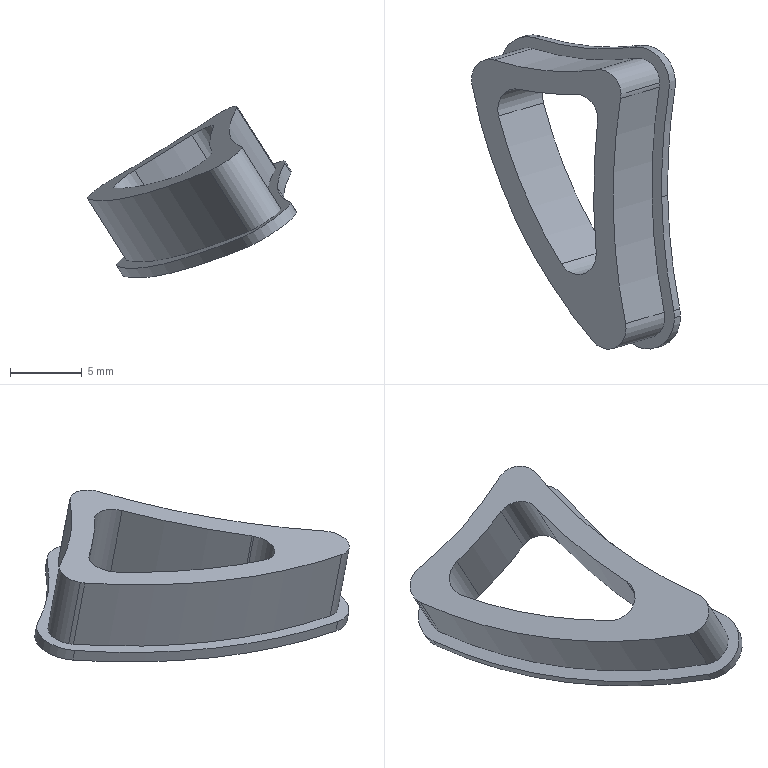Part | SolidWorks | features SplitBody 1 | 1 solid | 26 faces | box 14.584 x 21.952 x 12.002 mm | volume 557.744 mm3 | cylinder 23 | plane 3 | commonest cylinder face diameters 3.2 x9 4.8 x4 78.4 x2 43.2 x1 44.8 x1 48 x1
STEP:
#1=CARTESIAN_POINT('',(533.227,266.339,-385.084));
#2=VERTEX_POINT('',#1);
#3=CARTESIAN_POINT('',(533.176,266.825,-385.025));
#4=VERTEX_POINT('',#3);
#5=CARTESIAN_POINT('',(531.189,266.525,-386.337));
#6=DIRECTION('',(-0.5274,-0.157,0.835));
#7=DIRECTION('',(-0.8494,0.07732,-0.522));
#8=AXIS2_PLACEMENT_3D('',#5,#6,#7);
#9=CIRCLE('',#8,2.4);
#10=EDGE_CURVE('',#2,#4,#9,.T.);
#11=ORIENTED_EDGE('',*,*,#10,.F.);
#12=CARTESIAN_POINT('',(533.649,266.465,-385.752));
#13=VERTEX_POINT('',#12);
#14=CARTESIAN_POINT('',(533.649,266.465,-385.752));
#15=DIRECTION('',(0.5274,0.157,-0.835));
#16=VECTOR('',#15,1000.);
#17=LINE('',#14,#16);
#18=EDGE_CURVE('',#2,#13,#17,.T.);
#19=ORIENTED_EDGE('',*,*,#18,.T.);
#20=CARTESIAN_POINT('',(533.598,266.95,-385.693));
#21=VERTEX_POINT('',#20);
#22=CARTESIAN_POINT('',(531.611,266.65,-387.005));
#23=DIRECTION('',(0.5274,0.157,-0.835));
#24=DIRECTION('',(-0.8494,0.07732,-0.522));
#25=AXIS2_PLACEMENT_3D('',#22,#23,#24);
#26=CIRCLE('',#25,2.4);
#27=EDGE_CURVE('',#21,#13,#26,.T.);
#28=ORIENTED_EDGE('',*,*,#27,.F.);
#29=CARTESIAN_POINT('',(533.598,266.95,-385.693));
#30=DIRECTION('',(0.5274,0.157,-0.835));
#31=VECTOR('',#30,1000.);
#32=LINE('',#29,#31);
#33=EDGE_CURVE('',#4,#21,#32,.T.);
#34=ORIENTED_EDGE('',*,*,#33,.F.);
#35=EDGE_LOOP('',(#11,#19,#28,#34));
#36=FACE_OUTER_BOUND('',#35,.T.);
#37=CARTESIAN_POINT('',(531.611,266.65,-387.005));
#38=DIRECTION('',(0.5274,0.157,-0.835));
#39=DIRECTION('',(0.8494,-0.07732,0.522));
#40=AXIS2_PLACEMENT_3D('',#37,#38,#39);
#41=CYLINDRICAL_SURFACE('',#40,2.4);
#42=ADVANCED_FACE('',(#36),#41,.T.);
#43=CARTESIAN_POINT('',(529.493,281.935,-378.378));
#44=VERTEX_POINT('',#43);
#45=CARTESIAN_POINT('',(527.854,283.63,-379.094));
#46=VERTEX_POINT('',#45);
#47=CARTESIAN_POINT('',(528.134,282.059,-379.213));
#48=DIRECTION('',(-0.5274,-0.157,0.835));
#49=DIRECTION('',(-0.8494,0.07732,-0.522));
#50=AXIS2_PLACEMENT_3D('',#47,#48,#49);
#51=CIRCLE('',#50,1.6);
#52=EDGE_CURVE('',#44,#46,#51,.T.);
#53=ORIENTED_EDGE('',*,*,#52,.F.);
#54=CARTESIAN_POINT('',(532.193,282.739,-382.653));
#55=VERTEX_POINT('',#54);
#56=CARTESIAN_POINT('',(529.493,281.935,-378.378));
#57=DIRECTION('',(0.5274,0.157,-0.835));
#58=VECTOR('',#57,1000.);
#59=LINE('',#56,#58);
#60=EDGE_CURVE('',#44,#55,#59,.T.);
#61=ORIENTED_EDGE('',*,*,#60,.T.);
#62=CARTESIAN_POINT('',(530.555,284.434,-383.369));
#63=VERTEX_POINT('',#62);
#64=CARTESIAN_POINT('',(530.834,282.863,-383.488));
#65=DIRECTION('',(0.5274,0.157,-0.835));
#66=DIRECTION('',(-0.8494,0.07732,-0.522));
#67=AXIS2_PLACEMENT_3D('',#64,#65,#66);
#68=CIRCLE('',#67,1.6);
#69=EDGE_CURVE('',#63,#55,#68,.T.);
#70=ORIENTED_EDGE('',*,*,#69,.F.);
#71=CARTESIAN_POINT('',(527.854,283.63,-379.094));
#72=DIRECTION('',(0.5274,0.157,-0.835));
#73=VECTOR('',#72,1000.);
#74=LINE('',#71,#73);
#75=EDGE_CURVE('',#46,#63,#74,.T.);
#76=ORIENTED_EDGE('',*,*,#75,.F.);
#77=EDGE_LOOP('',(#53,#61,#70,#76));
#78=FACE_OUTER_BOUND('',#77,.T.);
#79=CARTESIAN_POINT('',(528.134,282.059,-379.213));
#80=DIRECTION('',(0.5274,0.157,-0.835));
#81=DIRECTION('',(0.8494,-0.07732,0.522));
#82=AXIS2_PLACEMENT_3D('',#79,#80,#81);
#83=CYLINDRICAL_SURFACE('',#82,1.6);
#84=ADVANCED_FACE('',(#78),#83,.T.);
#85=CARTESIAN_POINT('',(521.766,283.72,-389.055));
#86=VERTEX_POINT('',#85);
#87=CARTESIAN_POINT('',(523.36,285.118,-387.786));
#88=VERTEX_POINT('',#87);
#89=CARTESIAN_POINT('',(523.125,283.596,-388.22));
#90=DIRECTION('',(0.5274,0.157,-0.835));
#91=DIRECTION('',(-0.8494,0.07732,-0.522));
#92=AXIS2_PLACEMENT_3D('',#89,#90,#91);
#93=CIRCLE('',#92,1.6);
#94=EDGE_CURVE('',#86,#88,#93,.T.);
#95=ORIENTED_EDGE('',*,*,#94,.F.);
#96=CARTESIAN_POINT('',(519.066,282.916,-384.78));
#97=VERTEX_POINT('',#96);
#98=CARTESIAN_POINT('',(519.066,282.916,-384.78));
#99=DIRECTION('',(-0.5274,-0.157,0.835));
#100=VECTOR('',#99,1000.);
#101=LINE('',#98,#100);
#102=EDGE_CURVE('',#86,#97,#101,.T.);
#103=ORIENTED_EDGE('',*,*,#102,.T.);
#104=CARTESIAN_POINT('',(520.659,284.314,-383.511));
#105=VERTEX_POINT('',#104);
#106=CARTESIAN_POINT('',(520.425,282.792,-383.945));
#107=DIRECTION('',(-0.5274,-0.157,0.835));
#108=DIRECTION('',(-0.8494,0.07732,-0.522));
#109=AXIS2_PLACEMENT_3D('',#106,#107,#108);
#110=CIRCLE('',#109,1.6);
#111=EDGE_CURVE('',#105,#97,#110,.T.);
#112=ORIENTED_EDGE('',*,*,#111,.F.);
#113=CARTESIAN_POINT('',(520.659,284.314,-383.511));
#114=DIRECTION('',(-0.5274,-0.157,0.835));
#115=VECTOR('',#114,1000.);
#116=LINE('',#113,#115);
#117=EDGE_CURVE('',#88,#105,#116,.T.);
#118=ORIENTED_EDGE('',*,*,#117,.F.);
#119=EDGE_LOOP('',(#95,#103,#112,#118));
#120=FACE_OUTER_BOUND('',#119,.T.);
#121=CARTESIAN_POINT('',(520.425,282.792,-383.945));
#122=DIRECTION('',(-0.5274,-0.157,0.835));
#123=DIRECTION('',(-0.8494,0.07732,-0.522));
#124=AXIS2_PLACEMENT_3D('',#121,#122,#123);
#125=CYLINDRICAL_SURFACE('',#124,1.6);
#126=ADVANCED_FACE('',(#120),#125,.T.);
#127=CARTESIAN_POINT('',(527.769,270.804,-381.56));
#128=VERTEX_POINT('',#127);
#129=CARTESIAN_POINT('',(525.33,270.097,-383.234));
#130=VERTEX_POINT('',#129);
#131=CARTESIAN_POINT('',(526.41,270.928,-382.395));
#132=DIRECTION('',(0.5274,0.157,-0.835));
#133=DIRECTION('',(-0.8494,0.07732,-0.522));
#134=AXIS2_PLACEMENT_3D('',#131,#132,#133);
#135=CIRCLE('',#134,1.6);
#136=EDGE_CURVE('',#128,#130,#135,.T.);
#137=ORIENTED_EDGE('',*,*,#136,.F.);
#138=CARTESIAN_POINT('',(530.892,271.733,-386.503));
#139=VERTEX_POINT('',#138);
#140=CARTESIAN_POINT('',(527.769,270.804,-381.56));
#141=DIRECTION('',(0.5274,0.157,-0.835));
#142=VECTOR('',#141,1000.);
#143=LINE('',#140,#142);
#144=EDGE_CURVE('',#128,#139,#143,.T.);
#145=ORIENTED_EDGE('',*,*,#144,.T.);
#146=CARTESIAN_POINT('',(528.452,271.027,-388.177));
#147=VERTEX_POINT('',#146);
#148=CARTESIAN_POINT('',(529.533,271.857,-387.338));
#149=DIRECTION('',(-0.5274,-0.157,0.835));
#150=DIRECTION('',(-0.8494,0.07732,-0.522));
#151=AXIS2_PLACEMENT_3D('',#148,#149,#150);
#152=CIRCLE('',#151,1.6);
#153=EDGE_CURVE('',#147,#139,#152,.T.);
#154=ORIENTED_EDGE('',*,*,#153,.F.);
#155=CARTESIAN_POINT('',(525.33,270.097,-383.234));
#156=DIRECTION('',(0.5274,0.157,-0.835));
#157=VECTOR('',#156,1000.);
#158=LINE('',#155,#157);
#159=EDGE_CURVE('',#130,#147,#158,.T.);
#160=ORIENTED_EDGE('',*,*,#159,.F.);
#161=EDGE_LOOP('',(#137,#145,#154,#160));
#162=FACE_OUTER_BOUND('',#161,.T.);
#163=CARTESIAN_POINT('',(526.41,270.928,-382.395));
#164=DIRECTION('',(0.5274,0.157,-0.835));
#165=DIRECTION('',(0.8494,-0.07732,0.522));
#166=AXIS2_PLACEMENT_3D('',#163,#164,#165);
#167=CYLINDRICAL_SURFACE('',#166,1.6);
#168=ADVANCED_FACE('',(#162),#167,.F.);
#169=CARTESIAN_POINT('',(532.759,274.886,-384.731));
#170=VERTEX_POINT('',#169);
#171=CARTESIAN_POINT('',(566.056,271.855,-364.267));
#172=DIRECTION('',(0.5274,0.157,-0.835));
#173=DIRECTION('',(-0.8494,0.07732,-0.522));
#174=AXIS2_PLACEMENT_3D('',#171,#172,#173);
#175=CIRCLE('',#174,39.2);
#176=EDGE_CURVE('',#21,#170,#175,.T.);
#177=ORIENTED_EDGE('',*,*,#176,.T.);
#178=CARTESIAN_POINT('',(532.337,274.761,-384.063));
#179=VERTEX_POINT('',#178);
#180=CARTESIAN_POINT('',(532.759,274.886,-384.731));
#181=DIRECTION('',(-0.5274,-0.157,0.835));
#182=VECTOR('',#181,1000.);
#183=LINE('',#180,#182);
#184=EDGE_CURVE('',#170,#179,#183,.T.);
#185=ORIENTED_EDGE('',*,*,#184,.T.);
#186=CARTESIAN_POINT('',(565.634,271.73,-363.599));
#187=DIRECTION('',(0.5274,0.157,-0.835));
#188=DIRECTION('',(-0.8494,0.07732,-0.522));
#189=AXIS2_PLACEMENT_3D('',#186,#187,#188);
#190=CIRCLE('',#189,39.2);
#191=EDGE_CURVE('',#4,#179,#190,.T.);
#192=ORIENTED_EDGE('',*,*,#191,.F.);
#193=ORIENTED_EDGE('',*,*,#33,.T.);
#194=EDGE_LOOP('',(#177,#185,#192,#193));
#195=FACE_OUTER_BOUND('',#194,.T.);
#196=CARTESIAN_POINT('',(566.056,271.855,-364.267));
#197=DIRECTION('',(-0.5274,-0.157,0.835));
#198=DIRECTION('',(-0.8494,0.07732,-0.522));
#199=AXIS2_PLACEMENT_3D('',#196,#197,#198);
#200=CYLINDRICAL_SURFACE('',#199,39.2);
#201=ADVANCED_FACE('',(#195),#200,.F.);
#202=CARTESIAN_POINT('',(519.099,282.597,-384.819));
#203=VERTEX_POINT('',#202);
#204=CARTESIAN_POINT('',(527.566,264.672,-382.842));
#205=VERTEX_POINT('',#204);
#206=CARTESIAN_POINT('',(546.94,286.701,-366.461));
#207=DIRECTION('',(-0.5274,-0.157,0.835));
#208=DIRECTION('',(-0.8494,0.07732,-0.522));
#209=AXIS2_PLACEMENT_3D('',#206,#207,#208);
#210=CIRCLE('',#209,33.6);
#211=EDGE_CURVE('',#203,#205,#210,.T.);
#212=ORIENTED_EDGE('',*,*,#211,.F.);
#213=CARTESIAN_POINT('',(521.8,283.401,-389.094));
#214=VERTEX_POINT('',#213);
#215=CARTESIAN_POINT('',(519.099,282.597,-384.819));
#216=DIRECTION('',(0.5274,0.157,-0.835));
#217=VECTOR('',#216,1000.);
#218=LINE('',#215,#217);
#219=EDGE_CURVE('',#203,#214,#218,.T.);
#220=ORIENTED_EDGE('',*,*,#219,.T.);
#221=CARTESIAN_POINT('',(530.266,265.476,-387.117));
#222=VERTEX_POINT('',#221);
#223=CARTESIAN_POINT('',(549.64,287.505,-370.736));
#224=DIRECTION('',(-0.5274,-0.157,0.835));
#225=DIRECTION('',(-0.8494,0.07732,-0.522));
#226=AXIS2_PLACEMENT_3D('',#223,#224,#225);
#227=CIRCLE('',#226,33.6);
#228=EDGE_CURVE('',#214,#222,#227,.T.);
#229=ORIENTED_EDGE('',*,*,#228,.T.);
#230=CARTESIAN_POINT('',(527.566,264.672,-382.842));
#231=DIRECTION('',(-0.5274,-0.157,0.835));
#232=VECTOR('',#231,1000.);
#233=LINE('',#230,#232);
#234=EDGE_CURVE('',#222,#205,#233,.T.);
#235=ORIENTED_EDGE('',*,*,#234,.T.);
#236=EDGE_LOOP('',(#212,#220,#229,#235));
#237=FACE_OUTER_BOUND('',#236,.T.);
#238=CARTESIAN_POINT('',(546.94,286.701,-366.461));
#239=DIRECTION('',(0.5274,0.157,-0.835));
#240=DIRECTION('',(0.8494,-0.07732,0.522));
#241=AXIS2_PLACEMENT_3D('',#238,#239,#240);
#242=CYLINDRICAL_SURFACE('',#241,33.6);
#243=ADVANCED_FACE('',(#237),#242,.T.);
#244=CARTESIAN_POINT('',(532.514,266.725,-385.462));
#245=VERTEX_POINT('',#244);
#246=CARTESIAN_POINT('',(532.173,282.435,-382.723));
#247=VERTEX_POINT('',#246);
#248=CARTESIAN_POINT('',(565.634,271.73,-363.599));
#249=DIRECTION('',(0.5274,0.157,-0.835));
#250=DIRECTION('',(-0.8494,0.07732,-0.522));
#251=AXIS2_PLACEMENT_3D('',#248,#249,#250);
#252=CIRCLE('',#251,40.);
#253=EDGE_CURVE('',#245,#247,#252,.T.);
#254=ORIENTED_EDGE('',*,*,#253,.T.);
#255=CARTESIAN_POINT('',(529.472,281.631,-378.448));
#256=VERTEX_POINT('',#255);
#257=CARTESIAN_POINT('',(529.472,281.631,-378.448));
#258=DIRECTION('',(-0.5274,-0.157,0.835));
#259=VECTOR('',#258,1000.);
#260=LINE('',#257,#259);
#261=EDGE_CURVE('',#247,#256,#260,.T.);
#262=ORIENTED_EDGE('',*,*,#261,.T.);
#263=CARTESIAN_POINT('',(529.813,265.921,-381.187));
#264=VERTEX_POINT('',#263);
#265=CARTESIAN_POINT('',(562.933,270.926,-359.324));
#266=DIRECTION('',(0.5274,0.157,-0.835));
#267=DIRECTION('',(-0.8494,0.07732,-0.522));
#268=AXIS2_PLACEMENT_3D('',#265,#266,#267);
#269=CIRCLE('',#268,40.);
#270=EDGE_CURVE('',#264,#256,#269,.T.);
#271=ORIENTED_EDGE('',*,*,#270,.F.);
#272=CARTESIAN_POINT('',(529.813,265.921,-381.187));
#273=DIRECTION('',(0.5274,0.157,-0.835));
#274=VECTOR('',#273,1000.);
#275=LINE('',#272,#274);
#276=EDGE_CURVE('',#264,#245,#275,.T.);
#277=ORIENTED_EDGE('',*,*,#276,.T.);
#278=EDGE_LOOP('',(#254,#262,#271,#277));
#279=FACE_OUTER_BOUND('',#278,.T.);
#280=CARTESIAN_POINT('',(562.933,270.926,-359.324));
#281=DIRECTION('',(0.5274,0.157,-0.835));
#282=DIRECTION('',(0.8494,-0.07732,0.522));
#283=AXIS2_PLACEMENT_3D('',#280,#281,#282);
#284=CYLINDRICAL_SURFACE('',#283,40.);
#285=ADVANCED_FACE('',(#279),#284,.F.);
#286=CARTESIAN_POINT('',(529.473,282.854,-385.308));
#287=VERTEX_POINT('',#286);
#288=CARTESIAN_POINT('',(525.486,283.217,-387.758));
#289=VERTEX_POINT('',#288);
#290=CARTESIAN_POINT('',(527.063,306.552,-382.374));
#291=DIRECTION('',(0.5274,0.157,-0.835));
#292=DIRECTION('',(-0.8494,0.07732,-0.522));
#293=AXIS2_PLACEMENT_3D('',#290,#291,#292);
#294=CIRCLE('',#293,24.);
#295=EDGE_CURVE('',#287,#289,#294,.T.);
#296=ORIENTED_EDGE('',*,*,#295,.F.);
#297=CARTESIAN_POINT('',(526.351,281.925,-380.365));
#298=VERTEX_POINT('',#297);
#299=CARTESIAN_POINT('',(526.351,281.925,-380.365));
#300=DIRECTION('',(-0.5274,-0.157,0.835));
#301=VECTOR('',#300,1000.);
#302=LINE('',#299,#301);
#303=EDGE_CURVE('',#287,#298,#302,.T.);
#304=ORIENTED_EDGE('',*,*,#303,.T.);
#305=CARTESIAN_POINT('',(522.363,282.287,-382.815));
#306=VERTEX_POINT('',#305);
#307=CARTESIAN_POINT('',(523.941,305.622,-377.431));
#308=DIRECTION('',(0.5274,0.157,-0.835));
#309=DIRECTION('',(-0.8494,0.07732,-0.522));
#310=AXIS2_PLACEMENT_3D('',#307,#308,#309);
#311=CIRCLE('',#310,24.);
#312=EDGE_CURVE('',#298,#306,#311,.T.);
#313=ORIENTED_EDGE('',*,*,#312,.T.);
#314=CARTESIAN_POINT('',(522.363,282.287,-382.815));
#315=DIRECTION('',(0.5274,0.157,-0.835));
#316=VECTOR('',#315,1000.);
#317=LINE('',#314,#316);
#318=EDGE_CURVE('',#306,#289,#317,.T.);
#319=ORIENTED_EDGE('',*,*,#318,.T.);
#320=EDGE_LOOP('',(#296,#304,#313,#319));
#321=FACE_OUTER_BOUND('',#320,.T.);
#322=CARTESIAN_POINT('',(523.941,305.622,-377.431));
#323=DIRECTION('',(0.5274,0.157,-0.835));
#324=DIRECTION('',(0.8494,-0.07732,0.522));
#325=AXIS2_PLACEMENT_3D('',#322,#323,#324);
#326=CYLINDRICAL_SURFACE('',#325,24.);
#327=ADVANCED_FACE('',(#321),#326,.T.);
#328=CARTESIAN_POINT('',(530.885,271.857,-386.484));
#329=VERTEX_POINT('',#328);
#330=CARTESIAN_POINT('',(530.983,280.925,-384.717));
#331=VERTEX_POINT('',#330);
#332=CARTESIAN_POINT('',(566.056,271.855,-364.267));
#333=DIRECTION('',(0.5274,0.157,-0.835));
#334=DIRECTION('',(-0.8494,0.07732,-0.522));
#335=AXIS2_PLACEMENT_3D('',#332,#333,#334);
#336=CIRCLE('',#335,41.6);
#337=EDGE_CURVE('',#329,#331,#336,.T.);
#338=ORIENTED_EDGE('',*,*,#337,.F.);
#339=CARTESIAN_POINT('',(527.763,270.928,-381.541));
#340=VERTEX_POINT('',#339);
#341=CARTESIAN_POINT('',(527.763,270.928,-381.541));
#342=DIRECTION('',(-0.5274,-0.157,0.835));
#343=VECTOR('',#342,1000.);
#344=LINE('',#341,#343);
#345=EDGE_CURVE('',#329,#340,#344,.T.);
#346=ORIENTED_EDGE('',*,*,#345,.T.);
#347=CARTESIAN_POINT('',(527.861,279.996,-379.774));
#348=VERTEX_POINT('',#347);
#349=CARTESIAN_POINT('',(562.933,270.926,-359.324));
#350=DIRECTION('',(0.5274,0.157,-0.835));
#351=DIRECTION('',(-0.8494,0.07732,-0.522));
#352=AXIS2_PLACEMENT_3D('',#349,#350,#351);
#353=CIRCLE('',#352,41.6);
#354=EDGE_CURVE('',#340,#348,#353,.T.);
#355=ORIENTED_EDGE('',*,*,#354,.T.);
#356=CARTESIAN_POINT('',(527.861,279.996,-379.774));
#357=DIRECTION('',(0.5274,0.157,-0.835));
#358=VECTOR('',#357,1000.);
#359=LINE('',#356,#358);
#360=EDGE_CURVE('',#348,#331,#359,.T.);
#361=ORIENTED_EDGE('',*,*,#360,.T.);
#362=EDGE_LOOP('',(#338,#346,#355,#361));
#363=FACE_OUTER_BOUND('',#362,.T.);
#364=CARTESIAN_POINT('',(562.933,270.926,-359.324));
#365=DIRECTION('',(0.5274,0.157,-0.835));
#366=DIRECTION('',(0.8494,-0.07732,0.522));
#367=AXIS2_PLACEMENT_3D('',#364,#365,#366);
#368=CYLINDRICAL_SURFACE('',#367,41.6);
#369=ADVANCED_FACE('',(#363),#368,.T.);
#370=CARTESIAN_POINT('',(520.959,280.418,-384.054));
#371=VERTEX_POINT('',#370);
#372=CARTESIAN_POINT('',(546.94,286.701,-366.461));
#373=DIRECTION('',(-0.5274,-0.157,0.835));
#374=DIRECTION('',(-0.8494,0.07732,-0.522));
#375=AXIS2_PLACEMENT_3D('',#372,#373,#374);
#376=CIRCLE('',#375,32.);
#377=EDGE_CURVE('',#371,#130,#376,.T.);
#378=ORIENTED_EDGE('',*,*,#377,.T.);
#379=ORIENTED_EDGE('',*,*,#159,.T.);
#380=CARTESIAN_POINT('',(524.081,281.347,-388.997));
#381=VERTEX_POINT('',#380);
#382=CARTESIAN_POINT('',(550.062,287.63,-371.404));
#383=DIRECTION('',(-0.5274,-0.157,0.835));
#384=DIRECTION('',(-0.8494,0.07732,-0.522));
#385=AXIS2_PLACEMENT_3D('',#382,#383,#384);
#386=CIRCLE('',#385,32.);
#387=EDGE_CURVE('',#381,#147,#386,.T.);
#388=ORIENTED_EDGE('',*,*,#387,.F.);
#389=CARTESIAN_POINT('',(520.959,280.418,-384.054));
#390=DIRECTION('',(-0.5274,-0.157,0.835));
#391=VECTOR('',#390,1000.);
#392=LINE('',#389,#391);
#393=EDGE_CURVE('',#381,#371,#392,.T.);
#394=ORIENTED_EDGE('',*,*,#393,.T.);
#395=EDGE_LOOP('',(#378,#379,#388,#394));
#396=FACE_OUTER_BOUND('',#395,.T.);
#397=CARTESIAN_POINT('',(546.94,286.701,-366.461));
#398=DIRECTION('',(0.5274,0.157,-0.835));
#399=DIRECTION('',(0.8494,-0.07732,0.522));
#400=AXIS2_PLACEMENT_3D('',#397,#398,#399);
#401=CYLINDRICAL_SURFACE('',#400,32.);
#402=ADVANCED_FACE('',(#396),#401,.F.);
#403=CARTESIAN_POINT('',(526.641,306.426,-381.706));
#404=DIRECTION('',(0.5274,0.157,-0.835));
#405=DIRECTION('',(-0.8494,0.07732,-0.522));
#406=AXIS2_PLACEMENT_3D('',#403,#404,#405);
#407=CIRCLE('',#406,22.4);
#408=EDGE_CURVE('',#63,#88,#407,.T.);
#409=ORIENTED_EDGE('',*,*,#408,.T.);
#410=ORIENTED_EDGE('',*,*,#117,.T.);
#411=CARTESIAN_POINT('',(523.941,305.622,-377.431));
#412=DIRECTION('',(0.5274,0.157,-0.835));
#413=DIRECTION('',(-0.8494,0.07732,-0.522));
#414=AXIS2_PLACEMENT_3D('',#411,#412,#413);
#415=CIRCLE('',#414,22.4);
#416=EDGE_CURVE('',#46,#105,#415,.T.);
#417=ORIENTED_EDGE('',*,*,#416,.F.);
#418=ORIENTED_EDGE('',*,*,#75,.T.);
#419=EDGE_LOOP('',(#409,#410,#417,#418));
#420=FACE_OUTER_BOUND('',#419,.T.);
#421=CARTESIAN_POINT('',(523.941,305.622,-377.431));
#422=DIRECTION('',(0.5274,0.157,-0.835));
#423=DIRECTION('',(0.8494,-0.07732,0.522));
#424=AXIS2_PLACEMENT_3D('',#421,#422,#423);
#425=CYLINDRICAL_SURFACE('',#424,22.4);
#426=ADVANCED_FACE('',(#420),#425,.F.);
#427=ORIENTED_EDGE('',*,*,#312,.F.);
#428=CARTESIAN_POINT('',(526.512,280.345,-380.56));
#429=DIRECTION('',(0.5274,0.157,-0.835));
#430=DIRECTION('',(-0.8494,0.07732,-0.522));
#431=AXIS2_PLACEMENT_3D('',#428,#429,#430);
#432=CIRCLE('',#431,1.6);
#433=EDGE_CURVE('',#298,#348,#432,.T.);
#434=ORIENTED_EDGE('',*,*,#433,.T.);
#435=ORIENTED_EDGE('',*,*,#354,.F.);
#436=CARTESIAN_POINT('',(526.41,270.928,-382.395));
#437=DIRECTION('',(0.5274,0.157,-0.835));
#438=DIRECTION('',(-0.8494,0.07732,-0.522));
#439=AXIS2_PLACEMENT_3D('',#436,#437,#438);
#440=CIRCLE('',#439,1.6);
#441=EDGE_CURVE('',#340,#128,#440,.T.);
#442=ORIENTED_EDGE('',*,*,#441,.T.);
#443=ORIENTED_EDGE('',*,*,#136,.T.);
#444=ORIENTED_EDGE('',*,*,#377,.F.);
#445=CARTESIAN_POINT('',(522.258,280.732,-383.174));
#446=DIRECTION('',(0.5274,0.157,-0.835));
#447=DIRECTION('',(-0.8494,0.07732,-0.522));
#448=AXIS2_PLACEMENT_3D('',#445,#446,#447);
#449=CIRCLE('',#448,1.6);
#450=EDGE_CURVE('',#371,#306,#449,.T.);
#451=ORIENTED_EDGE('',*,*,#450,.T.);
#452=EDGE_LOOP('',(#427,#434,#435,#442,#443,#444,#451));
#453=FACE_BOUND('',#452,.T.);
#454=ORIENTED_EDGE('',*,*,#416,.T.);
#455=ORIENTED_EDGE('',*,*,#111,.T.);
#456=CARTESIAN_POINT('',(520.425,282.792,-383.945));
#457=DIRECTION('',(-0.5274,-0.157,0.835));
#458=DIRECTION('',(-0.8494,0.07732,-0.522));
#459=AXIS2_PLACEMENT_3D('',#456,#457,#458);
#460=CIRCLE('',#459,1.6);
#461=EDGE_CURVE('',#97,#203,#460,.T.);
#462=ORIENTED_EDGE('',*,*,#461,.T.);
#463=ORIENTED_EDGE('',*,*,#211,.T.);
#464=CARTESIAN_POINT('',(528.488,265.721,-382.062));
#465=DIRECTION('',(-0.5274,-0.157,0.835));
#466=DIRECTION('',(-0.8494,0.07732,-0.522));
#467=AXIS2_PLACEMENT_3D('',#464,#465,#466);
#468=CIRCLE('',#467,1.6);
#469=EDGE_CURVE('',#205,#264,#468,.T.);
#470=ORIENTED_EDGE('',*,*,#469,.T.);
#471=ORIENTED_EDGE('',*,*,#270,.T.);
#472=CARTESIAN_POINT('',(528.134,282.059,-379.213));
#473=DIRECTION('',(-0.5274,-0.157,0.835));
#474=DIRECTION('',(-0.8494,0.07732,-0.522));
#475=AXIS2_PLACEMENT_3D('',#472,#473,#474);
#476=CIRCLE('',#475,1.6);
#477=EDGE_CURVE('',#256,#44,#476,.T.);
#478=ORIENTED_EDGE('',*,*,#477,.T.);
#479=ORIENTED_EDGE('',*,*,#52,.T.);
#480=EDGE_LOOP('',(#454,#455,#462,#463,#470,#471,#478,#479));
#481=FACE_OUTER_BOUND('',#480,.T.);
#482=CARTESIAN_POINT('',(524.313,284.547,-381.159));
#483=DIRECTION('',(-0.5274,-0.157,0.835));
#484=DIRECTION('',(-0.8494,0.07732,-0.522));
#485=AXIS2_PLACEMENT_3D('',#482,#483,#484);
#486=PLANE('',#485);
#487=ADVANCED_FACE('',(#453,#481),#486,.T.);
#488=CARTESIAN_POINT('',(530.415,285.219,-383.31));
#489=VERTEX_POINT('',#488);
#490=CARTESIAN_POINT('',(523.477,285.879,-387.568));
#491=VERTEX_POINT('',#490);
#492=CARTESIAN_POINT('',(526.641,306.426,-381.706));
#493=DIRECTION('',(0.5274,0.157,-0.835));
#494=DIRECTION('',(-0.8494,0.07732,-0.522));
#495=AXIS2_PLACEMENT_3D('',#492,#493,#494);
#496=CIRCLE('',#495,21.6);
#497=EDGE_CURVE('',#489,#491,#496,.T.);
#498=ORIENTED_EDGE('',*,*,#497,.T.);
#499=CARTESIAN_POINT('',(521.137,283.303,-389.531));
#500=VERTEX_POINT('',#499);
#501=CARTESIAN_POINT('',(523.125,283.596,-388.22));
#502=DIRECTION('',(-0.5274,-0.157,0.835));
#503=DIRECTION('',(-0.8494,0.07732,-0.522));
#504=AXIS2_PLACEMENT_3D('',#501,#502,#503);
#505=CIRCLE('',#504,2.4);
#506=EDGE_CURVE('',#491,#500,#505,.T.);
#507=ORIENTED_EDGE('',*,*,#506,.T.);
#508=CARTESIAN_POINT('',(529.805,264.951,-387.507));
#509=VERTEX_POINT('',#508);
#510=CARTESIAN_POINT('',(549.64,287.505,-370.736));
#511=DIRECTION('',(-0.5274,-0.157,0.835));
#512=DIRECTION('',(-0.8494,0.07732,-0.522));
#513=AXIS2_PLACEMENT_3D('',#510,#511,#512);
#514=CIRCLE('',#513,34.4);
#515=EDGE_CURVE('',#500,#509,#514,.T.);
#516=ORIENTED_EDGE('',*,*,#515,.T.);
#517=CARTESIAN_POINT('',(531.189,266.525,-386.337));
#518=DIRECTION('',(-0.5274,-0.157,0.835));
#519=DIRECTION('',(-0.8494,0.07732,-0.522));
#520=AXIS2_PLACEMENT_3D('',#517,#518,#519);
#521=CIRCLE('',#520,2.4);
#522=EDGE_CURVE('',#509,#2,#521,.T.);
#523=ORIENTED_EDGE('',*,*,#522,.T.);
#524=ORIENTED_EDGE('',*,*,#10,.T.);
#525=ORIENTED_EDGE('',*,*,#191,.T.);
#526=CARTESIAN_POINT('',(532.842,282.22,-382.341));
#527=VERTEX_POINT('',#526);
#528=CARTESIAN_POINT('',(565.634,271.73,-363.599));
#529=DIRECTION('',(0.5274,0.157,-0.835));
#530=DIRECTION('',(-0.8494,0.07732,-0.522));
#531=AXIS2_PLACEMENT_3D('',#528,#529,#530);
#532=CIRCLE('',#531,39.2);
#533=EDGE_CURVE('',#179,#527,#532,.T.);
#534=ORIENTED_EDGE('',*,*,#533,.T.);
#535=CARTESIAN_POINT('',(530.834,282.863,-383.488));
#536=DIRECTION('',(-0.5274,-0.157,0.835));
#537=DIRECTION('',(-0.8494,0.07732,-0.522));
#538=AXIS2_PLACEMENT_3D('',#535,#536,#537);
#539=CIRCLE('',#538,2.4);
#540=EDGE_CURVE('',#527,#489,#539,.T.);
#541=ORIENTED_EDGE('',*,*,#540,.T.);
#542=EDGE_LOOP('',(#498,#507,#516,#523,#524,#525,#534,#541));
#543=FACE_OUTER_BOUND('',#542,.T.);
#544=ORIENTED_EDGE('',*,*,#228,.F.);
#545=CARTESIAN_POINT('',(523.125,283.596,-388.22));
#546=DIRECTION('',(0.5274,0.157,-0.835));
#547=DIRECTION('',(-0.8494,0.07732,-0.522));
#548=AXIS2_PLACEMENT_3D('',#545,#546,#547);
#549=CIRCLE('',#548,1.6);
#550=EDGE_CURVE('',#214,#86,#549,.T.);
#551=ORIENTED_EDGE('',*,*,#550,.T.);
#552=ORIENTED_EDGE('',*,*,#94,.T.);
#553=ORIENTED_EDGE('',*,*,#408,.F.);
#554=ORIENTED_EDGE('',*,*,#69,.T.);
#555=CARTESIAN_POINT('',(530.834,282.863,-383.488));
#556=DIRECTION('',(0.5274,0.157,-0.835));
#557=DIRECTION('',(-0.8494,0.07732,-0.522));
#558=AXIS2_PLACEMENT_3D('',#555,#556,#557);
#559=CIRCLE('',#558,1.6);
#560=EDGE_CURVE('',#55,#247,#559,.T.);
#561=ORIENTED_EDGE('',*,*,#560,.T.);
#562=ORIENTED_EDGE('',*,*,#253,.F.);
#563=CARTESIAN_POINT('',(531.189,266.525,-386.337));
#564=DIRECTION('',(0.5274,0.157,-0.835));
#565=DIRECTION('',(-0.8494,0.07732,-0.522));
#566=AXIS2_PLACEMENT_3D('',#563,#564,#565);
#567=CIRCLE('',#566,1.6);
#568=EDGE_CURVE('',#245,#222,#567,.T.);
#569=ORIENTED_EDGE('',*,*,#568,.T.);
#570=EDGE_LOOP('',(#544,#551,#552,#553,#554,#561,#562,#569));
#571=FACE_BOUND('',#570,.T.);
#572=CARTESIAN_POINT('',(527.014,285.351,-385.434));
#573=DIRECTION('',(-0.5274,-0.157,0.835));
#574=DIRECTION('',(-0.8494,0.07732,-0.522));
#575=AXIS2_PLACEMENT_3D('',#572,#573,#574);
#576=PLANE('',#575);
#577=ADVANCED_FACE('',(#543,#571),#576,.T.);
#578=ORIENTED_EDGE('',*,*,#184,.F.);
#579=CARTESIAN_POINT('',(533.264,282.346,-383.009));
#580=VERTEX_POINT('',#579);
#581=CARTESIAN_POINT('',(566.056,271.855,-364.267));
#582=DIRECTION('',(0.5274,0.157,-0.835));
#583=DIRECTION('',(-0.8494,0.07732,-0.522));
#584=AXIS2_PLACEMENT_3D('',#581,#582,#583);
#585=CIRCLE('',#584,39.2);
#586=EDGE_CURVE('',#170,#580,#585,.T.);
#587=ORIENTED_EDGE('',*,*,#586,.T.);
#588=CARTESIAN_POINT('',(533.264,282.346,-383.009));
#589=DIRECTION('',(-0.5274,-0.157,0.835));
#590=VECTOR('',#589,1000.);
#591=LINE('',#588,#590);
#592=EDGE_CURVE('',#580,#527,#591,.T.);
#593=ORIENTED_EDGE('',*,*,#592,.T.);
#594=ORIENTED_EDGE('',*,*,#533,.F.);
#595=EDGE_LOOP('',(#578,#587,#593,#594));
#596=FACE_OUTER_BOUND('',#595,.T.);
#597=CARTESIAN_POINT('',(566.056,271.855,-364.267));
#598=DIRECTION('',(-0.5274,-0.157,0.835));
#599=DIRECTION('',(-0.8494,0.07732,-0.522));
#600=AXIS2_PLACEMENT_3D('',#597,#598,#599);
#601=CYLINDRICAL_SURFACE('',#600,39.2);
#602=ADVANCED_FACE('',(#596),#601,.F.);
#603=ORIENTED_EDGE('',*,*,#515,.F.);
#604=CARTESIAN_POINT('',(521.559,283.429,-390.199));
#605=VERTEX_POINT('',#604);
#606=CARTESIAN_POINT('',(521.559,283.429,-390.199));
#607=DIRECTION('',(0.5274,0.157,-0.835));
#608=VECTOR('',#607,1000.);
#609=LINE('',#606,#608);
#610=EDGE_CURVE('',#500,#605,#609,.T.);
#611=ORIENTED_EDGE('',*,*,#610,.T.);
#612=CARTESIAN_POINT('',(530.227,265.077,-388.175));
#613=VERTEX_POINT('',#612);
#614=CARTESIAN_POINT('',(550.062,287.63,-371.404));
#615=DIRECTION('',(-0.5274,-0.157,0.835));
#616=DIRECTION('',(-0.8494,0.07732,-0.522));
#617=AXIS2_PLACEMENT_3D('',#614,#615,#616);
#618=CIRCLE('',#617,34.4);
#619=EDGE_CURVE('',#605,#613,#618,.T.);
#620=ORIENTED_EDGE('',*,*,#619,.T.);
#621=CARTESIAN_POINT('',(530.227,265.077,-388.175));
#622=DIRECTION('',(-0.5274,-0.157,0.835));
#623=VECTOR('',#622,1000.);
#624=LINE('',#621,#623);
#625=EDGE_CURVE('',#613,#509,#624,.T.);
#626=ORIENTED_EDGE('',*,*,#625,.T.);
#627=EDGE_LOOP('',(#603,#611,#620,#626));
#628=FACE_OUTER_BOUND('',#627,.T.);
#629=CARTESIAN_POINT('',(550.062,287.63,-371.404));
#630=DIRECTION('',(-0.5274,-0.157,0.835));
#631=DIRECTION('',(-0.8494,0.07732,-0.522));
#632=AXIS2_PLACEMENT_3D('',#629,#630,#631);
#633=CYLINDRICAL_SURFACE('',#632,34.4);
#634=ADVANCED_FACE('',(#628),#633,.T.);
#635=CARTESIAN_POINT('',(530.837,285.345,-383.978));
#636=VERTEX_POINT('',#635);
#637=CARTESIAN_POINT('',(523.899,286.005,-388.236));
#638=VERTEX_POINT('',#637);
#639=CARTESIAN_POINT('',(527.063,306.552,-382.374));
#640=DIRECTION('',(0.5274,0.157,-0.835));
#641=DIRECTION('',(-0.8494,0.07732,-0.522));
#642=AXIS2_PLACEMENT_3D('',#639,#640,#641);
#643=CIRCLE('',#642,21.6);
#644=EDGE_CURVE('',#636,#638,#643,.T.);
#645=ORIENTED_EDGE('',*,*,#644,.T.);
#646=CARTESIAN_POINT('',(523.899,286.005,-388.236));
#647=DIRECTION('',(-0.5274,-0.157,0.835));
#648=VECTOR('',#647,1000.);
#649=LINE('',#646,#648);
#650=EDGE_CURVE('',#638,#491,#649,.T.);
#651=ORIENTED_EDGE('',*,*,#650,.T.);
#652=ORIENTED_EDGE('',*,*,#497,.F.);
#653=CARTESIAN_POINT('',(530.837,285.345,-383.978));
#654=DIRECTION('',(0.5274,0.157,-0.835));
#655=VECTOR('',#654,1000.);
#656=LINE('',#653,#655);
#657=EDGE_CURVE('',#489,#636,#656,.T.);
#658=ORIENTED_EDGE('',*,*,#657,.T.);
#659=EDGE_LOOP('',(#645,#651,#652,#658));
#660=FACE_OUTER_BOUND('',#659,.T.);
#661=CARTESIAN_POINT('',(527.063,306.552,-382.374));
#662=DIRECTION('',(-0.5274,-0.157,0.835));
#663=DIRECTION('',(-0.8494,0.07732,-0.522));
#664=AXIS2_PLACEMENT_3D('',#661,#662,#663);
#665=CYLINDRICAL_SURFACE('',#664,21.6);
#666=ADVANCED_FACE('',(#660),#665,.F.);
#667=ORIENTED_EDGE('',*,*,#619,.F.);
#668=CARTESIAN_POINT('',(523.547,283.722,-388.888));
#669=DIRECTION('',(0.5274,0.157,-0.835));
#670=DIRECTION('',(-0.8494,0.07732,-0.522));
#671=AXIS2_PLACEMENT_3D('',#668,#669,#670);
#672=CIRCLE('',#671,2.4);
#673=EDGE_CURVE('',#605,#638,#672,.T.);
#674=ORIENTED_EDGE('',*,*,#673,.T.);
#675=ORIENTED_EDGE('',*,*,#644,.F.);
#676=CARTESIAN_POINT('',(531.256,282.988,-384.156));
#677=DIRECTION('',(0.5274,0.157,-0.835));
#678=DIRECTION('',(-0.8494,0.07732,-0.522));
#679=AXIS2_PLACEMENT_3D('',#676,#677,#678);
#680=CIRCLE('',#679,2.4);
#681=EDGE_CURVE('',#636,#580,#680,.T.);
#682=ORIENTED_EDGE('',*,*,#681,.T.);
#683=ORIENTED_EDGE('',*,*,#586,.F.);
#684=ORIENTED_EDGE('',*,*,#176,.F.);
#685=ORIENTED_EDGE('',*,*,#27,.T.);
#686=CARTESIAN_POINT('',(531.611,266.65,-387.005));
#687=DIRECTION('',(0.5274,0.157,-0.835));
#688=DIRECTION('',(-0.8494,0.07732,-0.522));
#689=AXIS2_PLACEMENT_3D('',#686,#687,#688);
#690=CIRCLE('',#689,2.4);
#691=EDGE_CURVE('',#13,#613,#690,.T.);
#692=ORIENTED_EDGE('',*,*,#691,.T.);
#693=EDGE_LOOP('',(#667,#674,#675,#682,#683,#684,#685,#692));
#694=FACE_OUTER_BOUND('',#693,.T.);
#695=ORIENTED_EDGE('',*,*,#337,.T.);
#696=CARTESIAN_POINT('',(529.634,281.274,-385.503));
#697=DIRECTION('',(-0.5274,-0.157,0.835));
#698=DIRECTION('',(-0.8494,0.07732,-0.522));
#699=AXIS2_PLACEMENT_3D('',#696,#697,#698);
#700=CIRCLE('',#699,1.6);
#701=EDGE_CURVE('',#331,#287,#700,.T.);
#702=ORIENTED_EDGE('',*,*,#701,.T.);
#703=ORIENTED_EDGE('',*,*,#295,.T.);
#704=CARTESIAN_POINT('',(525.38,281.661,-388.117));
#705=DIRECTION('',(-0.5274,-0.157,0.835));
#706=DIRECTION('',(-0.8494,0.07732,-0.522));
#707=AXIS2_PLACEMENT_3D('',#704,#705,#706);
#708=CIRCLE('',#707,1.6);
#709=EDGE_CURVE('',#289,#381,#708,.T.);
#710=ORIENTED_EDGE('',*,*,#709,.T.);
#711=ORIENTED_EDGE('',*,*,#387,.T.);
#712=ORIENTED_EDGE('',*,*,#153,.T.);
#713=CARTESIAN_POINT('',(529.533,271.857,-387.338));
#714=DIRECTION('',(-0.5274,-0.157,0.835));
#715=DIRECTION('',(-0.8494,0.07732,-0.522));
#716=AXIS2_PLACEMENT_3D('',#713,#714,#715);
#717=CIRCLE('',#716,1.6);
#718=EDGE_CURVE('',#139,#329,#717,.T.);
#719=ORIENTED_EDGE('',*,*,#718,.T.);
#720=EDGE_LOOP('',(#695,#702,#703,#710,#711,#712,#719));
#721=FACE_BOUND('',#720,.T.);
#722=CARTESIAN_POINT('',(527.436,285.477,-386.102));
#723=DIRECTION('',(-0.5274,-0.157,0.835));
#724=DIRECTION('',(-0.8494,0.07732,-0.522));
#725=AXIS2_PLACEMENT_3D('',#722,#723,#724);
#726=PLANE('',#725);
#727=ADVANCED_FACE('',(#694,#721),#726,.F.);
#728=ORIENTED_EDGE('',*,*,#469,.F.);
#729=ORIENTED_EDGE('',*,*,#234,.F.);
#730=ORIENTED_EDGE('',*,*,#568,.F.);
#731=ORIENTED_EDGE('',*,*,#276,.F.);
#732=EDGE_LOOP('',(#728,#729,#730,#731));
#733=FACE_OUTER_BOUND('',#732,.T.);
#734=CARTESIAN_POINT('',(528.488,265.721,-382.062));
#735=DIRECTION('',(-0.5274,-0.157,0.835));
#736=DIRECTION('',(-0.8494,0.07732,-0.522));
#737=AXIS2_PLACEMENT_3D('',#734,#735,#736);
#738=CYLINDRICAL_SURFACE('',#737,1.6);
#739=ADVANCED_FACE('',(#733),#738,.T.);
#740=ORIENTED_EDGE('',*,*,#144,.F.);
#741=ORIENTED_EDGE('',*,*,#441,.F.);
#742=ORIENTED_EDGE('',*,*,#345,.F.);
#743=ORIENTED_EDGE('',*,*,#718,.F.);
#744=EDGE_LOOP('',(#740,#741,#742,#743));
#745=FACE_OUTER_BOUND('',#744,.T.);
#746=CARTESIAN_POINT('',(526.41,270.928,-382.395));
#747=DIRECTION('',(0.5274,0.157,-0.835));
#748=DIRECTION('',(0.8494,-0.07732,0.522));
#749=AXIS2_PLACEMENT_3D('',#746,#747,#748);
#750=CYLINDRICAL_SURFACE('',#749,1.6);
#751=ADVANCED_FACE('',(#745),#750,.F.);
#752=ORIENTED_EDGE('',*,*,#433,.F.);
#753=ORIENTED_EDGE('',*,*,#303,.F.);
#754=ORIENTED_EDGE('',*,*,#701,.F.);
#755=ORIENTED_EDGE('',*,*,#360,.F.);
#756=EDGE_LOOP('',(#752,#753,#754,#755));
#757=FACE_OUTER_BOUND('',#756,.T.);
#758=CARTESIAN_POINT('',(526.512,280.345,-380.56));
#759=DIRECTION('',(-0.5274,-0.157,0.835));
#760=DIRECTION('',(-0.8494,0.07732,-0.522));
#761=AXIS2_PLACEMENT_3D('',#758,#759,#760);
#762=CYLINDRICAL_SURFACE('',#761,1.6);
#763=ADVANCED_FACE('',(#757),#762,.F.);
#764=ORIENTED_EDGE('',*,*,#450,.F.);
#765=ORIENTED_EDGE('',*,*,#393,.F.);
#766=ORIENTED_EDGE('',*,*,#709,.F.);
#767=ORIENTED_EDGE('',*,*,#318,.F.);
#768=EDGE_LOOP('',(#764,#765,#766,#767));
#769=FACE_OUTER_BOUND('',#768,.T.);
#770=CARTESIAN_POINT('',(522.258,280.732,-383.174));
#771=DIRECTION('',(0.5274,0.157,-0.835));
#772=DIRECTION('',(0.8494,-0.07732,0.522));
#773=AXIS2_PLACEMENT_3D('',#770,#771,#772);
#774=CYLINDRICAL_SURFACE('',#773,1.6);
#775=ADVANCED_FACE('',(#769),#774,.F.);
#776=ORIENTED_EDGE('',*,*,#102,.F.);
#777=ORIENTED_EDGE('',*,*,#550,.F.);
#778=ORIENTED_EDGE('',*,*,#219,.F.);
#779=ORIENTED_EDGE('',*,*,#461,.F.);
#780=EDGE_LOOP('',(#776,#777,#778,#779));
#781=FACE_OUTER_BOUND('',#780,.T.);
#782=CARTESIAN_POINT('',(520.425,282.792,-383.945));
#783=DIRECTION('',(-0.5274,-0.157,0.835));
#784=DIRECTION('',(-0.8494,0.07732,-0.522));
#785=AXIS2_PLACEMENT_3D('',#782,#783,#784);
#786=CYLINDRICAL_SURFACE('',#785,1.6);
#787=ADVANCED_FACE('',(#781),#786,.T.);
#788=ORIENTED_EDGE('',*,*,#60,.F.);
#789=ORIENTED_EDGE('',*,*,#477,.F.);
#790=ORIENTED_EDGE('',*,*,#261,.F.);
#791=ORIENTED_EDGE('',*,*,#560,.F.);
#792=EDGE_LOOP('',(#788,#789,#790,#791));
#793=FACE_OUTER_BOUND('',#792,.T.);
#794=CARTESIAN_POINT('',(528.134,282.059,-379.213));
#795=DIRECTION('',(0.5274,0.157,-0.835));
#796=DIRECTION('',(0.8494,-0.07732,0.522));
#797=AXIS2_PLACEMENT_3D('',#794,#795,#796);
#798=CYLINDRICAL_SURFACE('',#797,1.6);
#799=ADVANCED_FACE('',(#793),#798,.T.);
#800=ORIENTED_EDGE('',*,*,#673,.F.);
#801=ORIENTED_EDGE('',*,*,#610,.F.);
#802=ORIENTED_EDGE('',*,*,#506,.F.);
#803=ORIENTED_EDGE('',*,*,#650,.F.);
#804=EDGE_LOOP('',(#800,#801,#802,#803));
#805=FACE_OUTER_BOUND('',#804,.T.);
#806=CARTESIAN_POINT('',(523.547,283.722,-388.888));
#807=DIRECTION('',(0.5274,0.157,-0.835));
#808=DIRECTION('',(0.8494,-0.07732,0.522));
#809=AXIS2_PLACEMENT_3D('',#806,#807,#808);
#810=CYLINDRICAL_SURFACE('',#809,2.4);
#811=ADVANCED_FACE('',(#805),#810,.T.);
#812=ORIENTED_EDGE('',*,*,#681,.F.);
#813=ORIENTED_EDGE('',*,*,#657,.F.);
#814=ORIENTED_EDGE('',*,*,#540,.F.);
#815=ORIENTED_EDGE('',*,*,#592,.F.);
#816=EDGE_LOOP('',(#812,#813,#814,#815));
#817=FACE_OUTER_BOUND('',#816,.T.);
#818=CARTESIAN_POINT('',(531.256,282.988,-384.156));
#819=DIRECTION('',(-0.5274,-0.157,0.835));
#820=DIRECTION('',(-0.8494,0.07732,-0.522));
#821=AXIS2_PLACEMENT_3D('',#818,#819,#820);
#822=CYLINDRICAL_SURFACE('',#821,2.4);
#823=ADVANCED_FACE('',(#817),#822,.T.);
#824=ORIENTED_EDGE('',*,*,#18,.F.);
#825=ORIENTED_EDGE('',*,*,#522,.F.);
#826=ORIENTED_EDGE('',*,*,#625,.F.);
#827=ORIENTED_EDGE('',*,*,#691,.F.);
#828=EDGE_LOOP('',(#824,#825,#826,#827));
#829=FACE_OUTER_BOUND('',#828,.T.);
#830=CARTESIAN_POINT('',(531.611,266.65,-387.005));
#831=DIRECTION('',(0.5274,0.157,-0.835));
#832=DIRECTION('',(0.8494,-0.07732,0.522));
#833=AXIS2_PLACEMENT_3D('',#830,#831,#832);
#834=CYLINDRICAL_SURFACE('',#833,2.4);
#835=ADVANCED_FACE('',(#829),#834,.T.);
#836=CLOSED_SHELL('',(#42,#84,#126,#168,#201,#243,#285,#327,#369,#402,#426,#487,#577,#602,#634,#666,#727,#739,#751,#763,#775,#787,#799,#811,#823,#835));
#837=MANIFOLD_SOLID_BREP('',#836);
#838=CARTESIAN_POINT('',(0.,0.,0.));
#839=DIRECTION('',(0.,0.,1.));
#840=DIRECTION('',(1.,0.,0.));
#841=AXIS2_PLACEMENT_3D('',#838,#839,#840);
#842=(LENGTH_UNIT()NAMED_UNIT(*)SI_UNIT(.MILLI.,.METRE.));
#843=UNCERTAINTY_MEASURE_WITH_UNIT(LENGTH_MEASURE(0.00001),#842,'','');
#844=(NAMED_UNIT(*)PLANE_ANGLE_UNIT()SI_UNIT($,.RADIAN.));
#845=(NAMED_UNIT(*)SI_UNIT($,.STERADIAN.)SOLID_ANGLE_UNIT());
#846=(GEOMETRIC_REPRESENTATION_CONTEXT(3)GLOBAL_UNCERTAINTY_ASSIGNED_CONTEXT((#843))GLOBAL_UNIT_ASSIGNED_CONTEXT((#842,#844,#845))REPRESENTATION_CONTEXT('',''));
#847=ADVANCED_BREP_SHAPE_REPRESENTATION('',(#837,#841),#846);